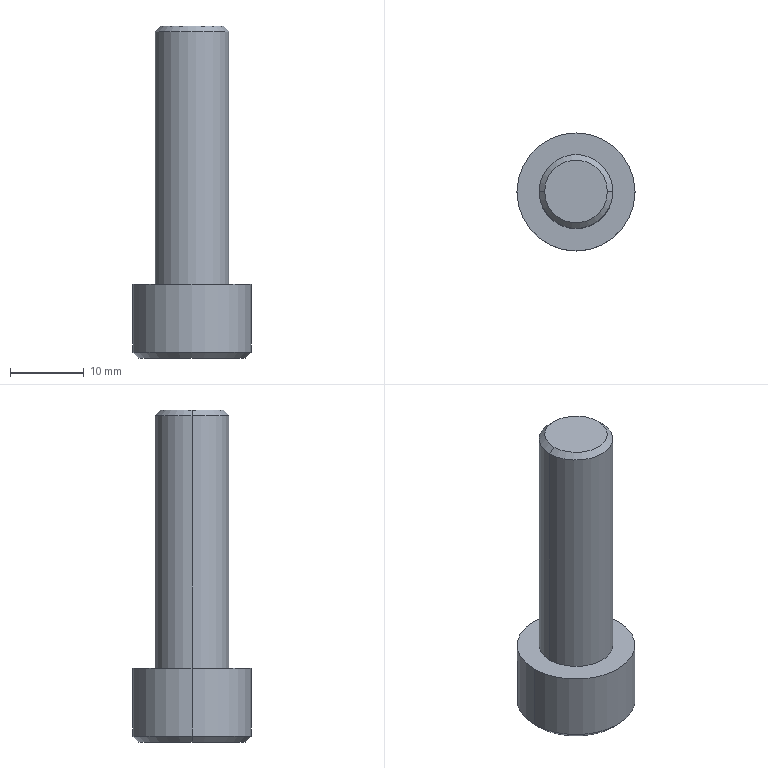Part | Creo | 1 solid | 18 faces | box 16 x 16 x 45 mm | volume 4403 mm3 | plane 10 | cylinder 4 | cone 4 | commonest cylinder face diameters 10 x2 16 x2
STEP:
#1=CARTESIAN_POINT('',(-123.202,226.324,-283.5));
#2=VERTEX_POINT('',#1);
#3=CARTESIAN_POINT('',(-107.202,226.324,-283.5));
#4=VERTEX_POINT('',#3);
#5=CARTESIAN_POINT('',(-115.202,226.324,-283.5));
#6=DIRECTION('',(0.,0.,1.));
#7=DIRECTION('',(-1.,0.,0.));
#8=AXIS2_PLACEMENT_3D('',#5,#6,#7);
#9=CIRCLE('',#8,8.);
#10=EDGE_CURVE('',#2,#4,#9,.T.);
#11=ORIENTED_EDGE('',*,*,#10,.F.);
#12=CARTESIAN_POINT('',(-115.202,226.324,-283.5));
#13=DIRECTION('',(0.,0.,1.));
#14=DIRECTION('',(1.,0.,0.));
#15=AXIS2_PLACEMENT_3D('',#12,#13,#14);
#16=CIRCLE('',#15,8.);
#17=EDGE_CURVE('',#4,#2,#16,.T.);
#18=ORIENTED_EDGE('',*,*,#17,.F.);
#19=EDGE_LOOP('',(#11,#18));
#20=FACE_OUTER_BOUND('',#19,.F.);
#21=CARTESIAN_POINT('',(-110.202,226.324,-283.5));
#22=VERTEX_POINT('',#21);
#23=CARTESIAN_POINT('',(-120.202,226.324,-283.5));
#24=VERTEX_POINT('',#23);
#25=CARTESIAN_POINT('',(-115.202,226.324,-283.5));
#26=DIRECTION('',(0.,0.,-1.));
#27=DIRECTION('',(1.,0.,0.));
#28=AXIS2_PLACEMENT_3D('',#25,#26,#27);
#29=CIRCLE('',#28,5.);
#30=EDGE_CURVE('',#22,#24,#29,.T.);
#31=ORIENTED_EDGE('',*,*,#30,.F.);
#32=CARTESIAN_POINT('',(-115.202,226.324,-283.5));
#33=DIRECTION('',(0.,0.,-1.));
#34=DIRECTION('',(-1.,0.,0.));
#35=AXIS2_PLACEMENT_3D('',#32,#33,#34);
#36=CIRCLE('',#35,5.);
#37=EDGE_CURVE('',#24,#22,#36,.T.);
#38=ORIENTED_EDGE('',*,*,#37,.F.);
#39=EDGE_LOOP('',(#31,#38));
#40=FACE_BOUND('',#39,.F.);
#41=CARTESIAN_POINT('',(-115.202,226.324,-283.5));
#42=DIRECTION('',(0.,0.,1.));
#43=DIRECTION('',(1.,0.,0.));
#44=AXIS2_PLACEMENT_3D('',#41,#42,#43);
#45=PLANE('',#44);
#46=ADVANCED_FACE('',(#20,#40),#45,.T.);
#47=CARTESIAN_POINT('',(-120.202,226.324,-249.25));
#48=VERTEX_POINT('',#47);
#49=CARTESIAN_POINT('',(-110.202,226.324,-249.25));
#50=VERTEX_POINT('',#49);
#51=CARTESIAN_POINT('',(-115.202,226.324,-249.25));
#52=DIRECTION('',(0.,0.,1.));
#53=DIRECTION('',(-1.,0.,0.));
#54=AXIS2_PLACEMENT_3D('',#51,#52,#53);
#55=CIRCLE('',#54,5.);
#56=EDGE_CURVE('',#48,#50,#55,.T.);
#57=ORIENTED_EDGE('',*,*,#56,.T.);
#58=CARTESIAN_POINT('',(-110.202,226.324,-283.5));
#59=DIRECTION('',(0.,0.,1.));
#60=VECTOR('',#59,34.25);
#61=LINE('',#58,#60);
#62=EDGE_CURVE('',#22,#50,#61,.T.);
#63=ORIENTED_EDGE('',*,*,#62,.F.);
#64=ORIENTED_EDGE('',*,*,#30,.T.);
#65=CARTESIAN_POINT('',(-120.202,226.324,-283.5));
#66=DIRECTION('',(0.,0.,1.));
#67=VECTOR('',#66,34.25);
#68=LINE('',#65,#67);
#69=EDGE_CURVE('',#24,#48,#68,.T.);
#70=ORIENTED_EDGE('',*,*,#69,.T.);
#71=EDGE_LOOP('',(#57,#63,#64,#70));
#72=FACE_OUTER_BOUND('',#71,.F.);
#73=CARTESIAN_POINT('',(-115.202,226.324,-295.5));
#74=DIRECTION('',(0.,0.,1.));
#75=DIRECTION('',(1.,0.,0.));
#76=AXIS2_PLACEMENT_3D('',#73,#74,#75);
#77=CYLINDRICAL_SURFACE('',#76,5.);
#78=ADVANCED_FACE('',(#72),#77,.T.);
#79=CARTESIAN_POINT('',(-119.452,226.324,-248.5));
#80=VERTEX_POINT('',#79);
#81=CARTESIAN_POINT('',(-110.952,226.324,-248.5));
#82=VERTEX_POINT('',#81);
#83=CARTESIAN_POINT('',(-115.202,226.324,-248.5));
#84=DIRECTION('',(0.,0.,1.));
#85=DIRECTION('',(-1.,0.,0.));
#86=AXIS2_PLACEMENT_3D('',#83,#84,#85);
#87=CIRCLE('',#86,4.25);
#88=EDGE_CURVE('',#80,#82,#87,.T.);
#89=ORIENTED_EDGE('',*,*,#88,.T.);
#90=CARTESIAN_POINT('',(-110.952,226.324,-248.5));
#91=DIRECTION('',(0.7071,0.,-0.7071));
#92=VECTOR('',#91,1.061);
#93=LINE('',#90,#92);
#94=EDGE_CURVE('',#82,#50,#93,.T.);
#95=ORIENTED_EDGE('',*,*,#94,.T.);
#96=ORIENTED_EDGE('',*,*,#56,.F.);
#97=CARTESIAN_POINT('',(-119.452,226.324,-248.5));
#98=DIRECTION('',(-0.7071,0.,-0.7071));
#99=VECTOR('',#98,1.061);
#100=LINE('',#97,#99);
#101=EDGE_CURVE('',#80,#48,#100,.T.);
#102=ORIENTED_EDGE('',*,*,#101,.F.);
#103=EDGE_LOOP('',(#89,#95,#96,#102));
#104=FACE_OUTER_BOUND('',#103,.F.);
#105=CARTESIAN_POINT('',(-115.202,226.324,-248.875));
#106=DIRECTION('',(0.,0.,-1.));
#107=DIRECTION('',(-1.,0.,0.));
#108=AXIS2_PLACEMENT_3D('',#105,#106,#107);
#109=CONICAL_SURFACE('',#108,4.625,45.);
#110=ADVANCED_FACE('',(#104),#109,.T.);
#111=CARTESIAN_POINT('',(-115.202,226.324,-248.5));
#112=DIRECTION('',(0.,0.,1.));
#113=DIRECTION('',(1.,0.,0.));
#114=AXIS2_PLACEMENT_3D('',#111,#112,#113);
#115=CIRCLE('',#114,4.25);
#116=EDGE_CURVE('',#82,#80,#115,.T.);
#117=ORIENTED_EDGE('',*,*,#116,.F.);
#118=ORIENTED_EDGE('',*,*,#88,.F.);
#119=EDGE_LOOP('',(#117,#118));
#120=FACE_OUTER_BOUND('',#119,.F.);
#121=CARTESIAN_POINT('',(-115.202,226.324,-248.5));
#122=DIRECTION('',(0.,0.,1.));
#123=DIRECTION('',(1.,0.,0.));
#124=AXIS2_PLACEMENT_3D('',#121,#122,#123);
#125=PLANE('',#124);
#126=ADVANCED_FACE('',(#120),#125,.T.);
#127=ORIENTED_EDGE('',*,*,#116,.T.);
#128=ORIENTED_EDGE('',*,*,#101,.T.);
#129=CARTESIAN_POINT('',(-115.202,226.324,-249.25));
#130=DIRECTION('',(0.,0.,1.));
#131=DIRECTION('',(1.,0.,0.));
#132=AXIS2_PLACEMENT_3D('',#129,#130,#131);
#133=CIRCLE('',#132,5.);
#134=EDGE_CURVE('',#50,#48,#133,.T.);
#135=ORIENTED_EDGE('',*,*,#134,.F.);
#136=ORIENTED_EDGE('',*,*,#94,.F.);
#137=EDGE_LOOP('',(#127,#128,#135,#136));
#138=FACE_OUTER_BOUND('',#137,.F.);
#139=CARTESIAN_POINT('',(-115.202,226.324,-248.875));
#140=DIRECTION('',(0.,0.,-1.));
#141=DIRECTION('',(-1.,0.,0.));
#142=AXIS2_PLACEMENT_3D('',#139,#140,#141);
#143=CONICAL_SURFACE('',#142,4.625,45.);
#144=ADVANCED_FACE('',(#138),#143,.T.);
#145=ORIENTED_EDGE('',*,*,#134,.T.);
#146=ORIENTED_EDGE('',*,*,#69,.F.);
#147=ORIENTED_EDGE('',*,*,#37,.T.);
#148=ORIENTED_EDGE('',*,*,#62,.T.);
#149=EDGE_LOOP('',(#145,#146,#147,#148));
#150=FACE_OUTER_BOUND('',#149,.F.);
#151=CARTESIAN_POINT('',(-115.202,226.324,-295.5));
#152=DIRECTION('',(0.,0.,1.));
#153=DIRECTION('',(1.,0.,0.));
#154=AXIS2_PLACEMENT_3D('',#151,#152,#153);
#155=CYLINDRICAL_SURFACE('',#154,5.);
#156=ADVANCED_FACE('',(#150),#155,.T.);
#157=CARTESIAN_POINT('',(-107.202,226.324,-292.7));
#158=VERTEX_POINT('',#157);
#159=CARTESIAN_POINT('',(-123.202,226.324,-292.7));
#160=VERTEX_POINT('',#159);
#161=CARTESIAN_POINT('',(-115.202,226.324,-292.7));
#162=DIRECTION('',(0.,0.,-1.));
#163=DIRECTION('',(1.,0.,0.));
#164=AXIS2_PLACEMENT_3D('',#161,#162,#163);
#165=CIRCLE('',#164,8.);
#166=EDGE_CURVE('',#158,#160,#165,.T.);
#167=ORIENTED_EDGE('',*,*,#166,.T.);
#168=CARTESIAN_POINT('',(-123.202,226.324,-292.7));
#169=DIRECTION('',(0.,0.,1.));
#170=VECTOR('',#169,9.2);
#171=LINE('',#168,#170);
#172=EDGE_CURVE('',#160,#2,#171,.T.);
#173=ORIENTED_EDGE('',*,*,#172,.T.);
#174=ORIENTED_EDGE('',*,*,#10,.T.);
#175=CARTESIAN_POINT('',(-107.202,226.324,-292.7));
#176=DIRECTION('',(0.,0.,1.));
#177=VECTOR('',#176,9.2);
#178=LINE('',#175,#177);
#179=EDGE_CURVE('',#158,#4,#178,.T.);
#180=ORIENTED_EDGE('',*,*,#179,.F.);
#181=EDGE_LOOP('',(#167,#173,#174,#180));
#182=FACE_OUTER_BOUND('',#181,.F.);
#183=CARTESIAN_POINT('',(-115.202,226.324,-295.5));
#184=DIRECTION('',(0.,0.,1.));
#185=DIRECTION('',(1.,0.,0.));
#186=AXIS2_PLACEMENT_3D('',#183,#184,#185);
#187=CYLINDRICAL_SURFACE('',#186,8.);
#188=ADVANCED_FACE('',(#182),#187,.T.);
#189=CARTESIAN_POINT('',(-108.002,226.324,-293.5));
#190=VERTEX_POINT('',#189);
#191=CARTESIAN_POINT('',(-122.402,226.324,-293.5));
#192=VERTEX_POINT('',#191);
#193=CARTESIAN_POINT('',(-115.202,226.324,-293.5));
#194=DIRECTION('',(0.,0.,-1.));
#195=DIRECTION('',(1.,0.,0.));
#196=AXIS2_PLACEMENT_3D('',#193,#194,#195);
#197=CIRCLE('',#196,7.2);
#198=EDGE_CURVE('',#190,#192,#197,.T.);
#199=ORIENTED_EDGE('',*,*,#198,.T.);
#200=CARTESIAN_POINT('',(-122.402,226.324,-293.5));
#201=DIRECTION('',(-0.7071,0.,0.7071));
#202=VECTOR('',#201,1.131);
#203=LINE('',#200,#202);
#204=EDGE_CURVE('',#192,#160,#203,.T.);
#205=ORIENTED_EDGE('',*,*,#204,.T.);
#206=ORIENTED_EDGE('',*,*,#166,.F.);
#207=CARTESIAN_POINT('',(-108.002,226.324,-293.5));
#208=DIRECTION('',(0.7071,0.,0.7071));
#209=VECTOR('',#208,1.131);
#210=LINE('',#207,#209);
#211=EDGE_CURVE('',#190,#158,#210,.T.);
#212=ORIENTED_EDGE('',*,*,#211,.F.);
#213=EDGE_LOOP('',(#199,#205,#206,#212));
#214=FACE_OUTER_BOUND('',#213,.F.);
#215=CARTESIAN_POINT('',(-115.202,226.324,-293.1));
#216=DIRECTION('',(0.,0.,1.));
#217=DIRECTION('',(1.,0.,0.));
#218=AXIS2_PLACEMENT_3D('',#215,#216,#217);
#219=CONICAL_SURFACE('',#218,7.6,45.);
#220=ADVANCED_FACE('',(#214),#219,.T.);
#221=ORIENTED_EDGE('',*,*,#198,.F.);
#222=CARTESIAN_POINT('',(-115.202,226.324,-293.5));
#223=DIRECTION('',(0.,0.,-1.));
#224=DIRECTION('',(-1.,0.,0.));
#225=AXIS2_PLACEMENT_3D('',#222,#223,#224);
#226=CIRCLE('',#225,7.2);
#227=EDGE_CURVE('',#192,#190,#226,.T.);
#228=ORIENTED_EDGE('',*,*,#227,.F.);
#229=EDGE_LOOP('',(#221,#228));
#230=FACE_OUTER_BOUND('',#229,.F.);
#231=CARTESIAN_POINT('',(-119.202,224.014,-293.5));
#232=VERTEX_POINT('',#231);
#233=CARTESIAN_POINT('',(-115.202,221.705,-293.5));
#234=VERTEX_POINT('',#233);
#235=CARTESIAN_POINT('',(-119.202,224.014,-293.5));
#236=DIRECTION('',(0.866,-0.5,0.));
#237=VECTOR('',#236,4.619);
#238=LINE('',#235,#237);
#239=EDGE_CURVE('',#232,#234,#238,.T.);
#240=ORIENTED_EDGE('',*,*,#239,.F.);
#241=CARTESIAN_POINT('',(-119.202,228.633,-293.5));
#242=VERTEX_POINT('',#241);
#243=CARTESIAN_POINT('',(-119.202,228.633,-293.5));
#244=DIRECTION('',(0.,-1.,0.));
#245=VECTOR('',#244,4.619);
#246=LINE('',#243,#245);
#247=EDGE_CURVE('',#242,#232,#246,.T.);
#248=ORIENTED_EDGE('',*,*,#247,.F.);
#249=CARTESIAN_POINT('',(-115.202,230.943,-293.5));
#250=VERTEX_POINT('',#249);
#251=CARTESIAN_POINT('',(-115.202,230.943,-293.5));
#252=DIRECTION('',(-0.866,-0.5,0.));
#253=VECTOR('',#252,4.619);
#254=LINE('',#251,#253);
#255=EDGE_CURVE('',#250,#242,#254,.T.);
#256=ORIENTED_EDGE('',*,*,#255,.F.);
#257=CARTESIAN_POINT('',(-111.202,228.633,-293.5));
#258=VERTEX_POINT('',#257);
#259=CARTESIAN_POINT('',(-111.202,228.633,-293.5));
#260=DIRECTION('',(-0.866,0.5,0.));
#261=VECTOR('',#260,4.619);
#262=LINE('',#259,#261);
#263=EDGE_CURVE('',#258,#250,#262,.T.);
#264=ORIENTED_EDGE('',*,*,#263,.F.);
#265=CARTESIAN_POINT('',(-111.202,224.014,-293.5));
#266=VERTEX_POINT('',#265);
#267=CARTESIAN_POINT('',(-111.202,224.014,-293.5));
#268=DIRECTION('',(0.,1.,0.));
#269=VECTOR('',#268,4.619);
#270=LINE('',#267,#269);
#271=EDGE_CURVE('',#266,#258,#270,.T.);
#272=ORIENTED_EDGE('',*,*,#271,.F.);
#273=CARTESIAN_POINT('',(-115.202,221.705,-293.5));
#274=DIRECTION('',(0.866,0.5,0.));
#275=VECTOR('',#274,4.619);
#276=LINE('',#273,#275);
#277=EDGE_CURVE('',#234,#266,#276,.T.);
#278=ORIENTED_EDGE('',*,*,#277,.F.);
#279=EDGE_LOOP('',(#240,#248,#256,#264,#272,#278));
#280=FACE_BOUND('',#279,.F.);
#281=CARTESIAN_POINT('',(-115.202,226.324,-293.5));
#282=DIRECTION('',(0.,0.,1.));
#283=DIRECTION('',(1.,0.,0.));
#284=AXIS2_PLACEMENT_3D('',#281,#282,#283);
#285=PLANE('',#284);
#286=ADVANCED_FACE('',(#230,#280),#285,.F.);
#287=ORIENTED_EDGE('',*,*,#227,.T.);
#288=ORIENTED_EDGE('',*,*,#211,.T.);
#289=CARTESIAN_POINT('',(-115.202,226.324,-292.7));
#290=DIRECTION('',(0.,0.,-1.));
#291=DIRECTION('',(-1.,0.,0.));
#292=AXIS2_PLACEMENT_3D('',#289,#290,#291);
#293=CIRCLE('',#292,8.);
#294=EDGE_CURVE('',#160,#158,#293,.T.);
#295=ORIENTED_EDGE('',*,*,#294,.F.);
#296=ORIENTED_EDGE('',*,*,#204,.F.);
#297=EDGE_LOOP('',(#287,#288,#295,#296));
#298=FACE_OUTER_BOUND('',#297,.F.);
#299=CARTESIAN_POINT('',(-115.202,226.324,-293.1));
#300=DIRECTION('',(0.,0.,1.));
#301=DIRECTION('',(1.,0.,0.));
#302=AXIS2_PLACEMENT_3D('',#299,#300,#301);
#303=CONICAL_SURFACE('',#302,7.6,45.);
#304=ADVANCED_FACE('',(#298),#303,.T.);
#305=ORIENTED_EDGE('',*,*,#294,.T.);
#306=ORIENTED_EDGE('',*,*,#179,.T.);
#307=ORIENTED_EDGE('',*,*,#17,.T.);
#308=ORIENTED_EDGE('',*,*,#172,.F.);
#309=EDGE_LOOP('',(#305,#306,#307,#308));
#310=FACE_OUTER_BOUND('',#309,.F.);
#311=CARTESIAN_POINT('',(-115.202,226.324,-295.5));
#312=DIRECTION('',(0.,0.,1.));
#313=DIRECTION('',(1.,0.,0.));
#314=AXIS2_PLACEMENT_3D('',#311,#312,#313);
#315=CYLINDRICAL_SURFACE('',#314,8.);
#316=ADVANCED_FACE('',(#310),#315,.T.);
#317=ORIENTED_EDGE('',*,*,#239,.T.);
#318=CARTESIAN_POINT('',(-115.202,221.705,-287.5));
#319=VERTEX_POINT('',#318);
#320=CARTESIAN_POINT('',(-115.202,221.705,-293.5));
#321=DIRECTION('',(0.,0.,1.));
#322=VECTOR('',#321,6.);
#323=LINE('',#320,#322);
#324=EDGE_CURVE('',#234,#319,#323,.T.);
#325=ORIENTED_EDGE('',*,*,#324,.T.);
#326=CARTESIAN_POINT('',(-119.202,224.014,-287.5));
#327=VERTEX_POINT('',#326);
#328=CARTESIAN_POINT('',(-115.202,221.705,-287.5));
#329=DIRECTION('',(-0.866,0.5,0.));
#330=VECTOR('',#329,4.619);
#331=LINE('',#328,#330);
#332=EDGE_CURVE('',#319,#327,#331,.T.);
#333=ORIENTED_EDGE('',*,*,#332,.T.);
#334=CARTESIAN_POINT('',(-119.202,224.014,-293.5));
#335=DIRECTION('',(0.,0.,1.));
#336=VECTOR('',#335,6.);
#337=LINE('',#334,#336);
#338=EDGE_CURVE('',#232,#327,#337,.T.);
#339=ORIENTED_EDGE('',*,*,#338,.F.);
#340=EDGE_LOOP('',(#317,#325,#333,#339));
#341=FACE_OUTER_BOUND('',#340,.F.);
#342=CARTESIAN_POINT('',(-115.202,221.705,-287.5));
#343=DIRECTION('',(-0.5,-0.866,0.));
#344=DIRECTION('',(0.866,-0.5,0.));
#345=AXIS2_PLACEMENT_3D('',#342,#343,#344);
#346=PLANE('',#345);
#347=ADVANCED_FACE('',(#341),#346,.F.);
#348=ORIENTED_EDGE('',*,*,#277,.T.);
#349=CARTESIAN_POINT('',(-111.202,224.014,-287.5));
#350=VERTEX_POINT('',#349);
#351=CARTESIAN_POINT('',(-111.202,224.014,-293.5));
#352=DIRECTION('',(0.,0.,1.));
#353=VECTOR('',#352,6.);
#354=LINE('',#351,#353);
#355=EDGE_CURVE('',#266,#350,#354,.T.);
#356=ORIENTED_EDGE('',*,*,#355,.T.);
#357=CARTESIAN_POINT('',(-111.202,224.014,-287.5));
#358=DIRECTION('',(-0.866,-0.5,0.));
#359=VECTOR('',#358,4.619);
#360=LINE('',#357,#359);
#361=EDGE_CURVE('',#350,#319,#360,.T.);
#362=ORIENTED_EDGE('',*,*,#361,.T.);
#363=ORIENTED_EDGE('',*,*,#324,.F.);
#364=EDGE_LOOP('',(#348,#356,#362,#363));
#365=FACE_OUTER_BOUND('',#364,.F.);
#366=CARTESIAN_POINT('',(-111.202,224.014,-287.5));
#367=DIRECTION('',(0.5,-0.866,0.));
#368=DIRECTION('',(0.866,0.5,0.));
#369=AXIS2_PLACEMENT_3D('',#366,#367,#368);
#370=PLANE('',#369);
#371=ADVANCED_FACE('',(#365),#370,.F.);
#372=ORIENTED_EDGE('',*,*,#271,.T.);
#373=CARTESIAN_POINT('',(-111.202,228.633,-287.5));
#374=VERTEX_POINT('',#373);
#375=CARTESIAN_POINT('',(-111.202,228.633,-293.5));
#376=DIRECTION('',(0.,0.,1.));
#377=VECTOR('',#376,6.);
#378=LINE('',#375,#377);
#379=EDGE_CURVE('',#258,#374,#378,.T.);
#380=ORIENTED_EDGE('',*,*,#379,.T.);
#381=CARTESIAN_POINT('',(-111.202,224.014,-287.5));
#382=DIRECTION('',(0.,1.,0.));
#383=VECTOR('',#382,4.619);
#384=LINE('',#381,#383);
#385=EDGE_CURVE('',#350,#374,#384,.T.);
#386=ORIENTED_EDGE('',*,*,#385,.F.);
#387=ORIENTED_EDGE('',*,*,#355,.F.);
#388=EDGE_LOOP('',(#372,#380,#386,#387));
#389=FACE_OUTER_BOUND('',#388,.F.);
#390=CARTESIAN_POINT('',(-111.202,228.633,-287.5));
#391=DIRECTION('',(1.,0.,0.));
#392=DIRECTION('',(0.,0.,-1.));
#393=AXIS2_PLACEMENT_3D('',#390,#391,#392);
#394=PLANE('',#393);
#395=ADVANCED_FACE('',(#389),#394,.F.);
#396=ORIENTED_EDGE('',*,*,#263,.T.);
#397=CARTESIAN_POINT('',(-115.202,230.943,-287.5));
#398=VERTEX_POINT('',#397);
#399=CARTESIAN_POINT('',(-115.202,230.943,-293.5));
#400=DIRECTION('',(0.,0.,1.));
#401=VECTOR('',#400,6.);
#402=LINE('',#399,#401);
#403=EDGE_CURVE('',#250,#398,#402,.T.);
#404=ORIENTED_EDGE('',*,*,#403,.T.);
#405=CARTESIAN_POINT('',(-115.202,230.943,-287.5));
#406=DIRECTION('',(0.866,-0.5,0.));
#407=VECTOR('',#406,4.619);
#408=LINE('',#405,#407);
#409=EDGE_CURVE('',#398,#374,#408,.T.);
#410=ORIENTED_EDGE('',*,*,#409,.T.);
#411=ORIENTED_EDGE('',*,*,#379,.F.);
#412=EDGE_LOOP('',(#396,#404,#410,#411));
#413=FACE_OUTER_BOUND('',#412,.F.);
#414=CARTESIAN_POINT('',(-115.202,230.943,-287.5));
#415=DIRECTION('',(0.5,0.866,0.));
#416=DIRECTION('',(-0.866,0.5,0.));
#417=AXIS2_PLACEMENT_3D('',#414,#415,#416);
#418=PLANE('',#417);
#419=ADVANCED_FACE('',(#413),#418,.F.);
#420=ORIENTED_EDGE('',*,*,#255,.T.);
#421=CARTESIAN_POINT('',(-119.202,228.633,-287.5));
#422=VERTEX_POINT('',#421);
#423=CARTESIAN_POINT('',(-119.202,228.633,-293.5));
#424=DIRECTION('',(0.,0.,1.));
#425=VECTOR('',#424,6.);
#426=LINE('',#423,#425);
#427=EDGE_CURVE('',#242,#422,#426,.T.);
#428=ORIENTED_EDGE('',*,*,#427,.T.);
#429=CARTESIAN_POINT('',(-119.202,228.633,-287.5));
#430=DIRECTION('',(0.866,0.5,0.));
#431=VECTOR('',#430,4.619);
#432=LINE('',#429,#431);
#433=EDGE_CURVE('',#422,#398,#432,.T.);
#434=ORIENTED_EDGE('',*,*,#433,.T.);
#435=ORIENTED_EDGE('',*,*,#403,.F.);
#436=EDGE_LOOP('',(#420,#428,#434,#435));
#437=FACE_OUTER_BOUND('',#436,.F.);
#438=CARTESIAN_POINT('',(-119.202,228.633,-287.5));
#439=DIRECTION('',(-0.5,0.866,0.));
#440=DIRECTION('',(-0.866,-0.5,0.));
#441=AXIS2_PLACEMENT_3D('',#438,#439,#440);
#442=PLANE('',#441);
#443=ADVANCED_FACE('',(#437),#442,.F.);
#444=ORIENTED_EDGE('',*,*,#247,.T.);
#445=ORIENTED_EDGE('',*,*,#338,.T.);
#446=CARTESIAN_POINT('',(-119.202,228.633,-287.5));
#447=DIRECTION('',(0.,-1.,0.));
#448=VECTOR('',#447,4.619);
#449=LINE('',#446,#448);
#450=EDGE_CURVE('',#422,#327,#449,.T.);
#451=ORIENTED_EDGE('',*,*,#450,.F.);
#452=ORIENTED_EDGE('',*,*,#427,.F.);
#453=EDGE_LOOP('',(#444,#445,#451,#452));
#454=FACE_OUTER_BOUND('',#453,.F.);
#455=CARTESIAN_POINT('',(-119.202,224.014,-287.5));
#456=DIRECTION('',(-1.,0.,0.));
#457=DIRECTION('',(0.,0.,1.));
#458=AXIS2_PLACEMENT_3D('',#455,#456,#457);
#459=PLANE('',#458);
#460=ADVANCED_FACE('',(#454),#459,.F.);
#461=ORIENTED_EDGE('',*,*,#361,.F.);
#462=ORIENTED_EDGE('',*,*,#385,.T.);
#463=ORIENTED_EDGE('',*,*,#409,.F.);
#464=ORIENTED_EDGE('',*,*,#433,.F.);
#465=ORIENTED_EDGE('',*,*,#450,.T.);
#466=ORIENTED_EDGE('',*,*,#332,.F.);
#467=EDGE_LOOP('',(#461,#462,#463,#464,#465,#466));
#468=FACE_OUTER_BOUND('',#467,.F.);
#469=CARTESIAN_POINT('',(-115.202,221.705,-287.5));
#470=DIRECTION('',(0.,0.,-1.));
#471=DIRECTION('',(-1.,0.,0.));
#472=AXIS2_PLACEMENT_3D('',#469,#470,#471);
#473=PLANE('',#472);
#474=ADVANCED_FACE('',(#468),#473,.T.);
#475=CLOSED_SHELL('',(#46,#78,#110,#126,#144,#156,#188,#220,#286,#304,#316,#347,#371,#395,#419,#443,#460,#474));
#476=MANIFOLD_SOLID_BREP('',#475);
#477=(LENGTH_UNIT()NAMED_UNIT(*)SI_UNIT(.MILLI.,.METRE.));
#478=UNCERTAINTY_MEASURE_WITH_UNIT(LENGTH_MEASURE(0.005037),#477,'','');
#479=(NAMED_UNIT(*)PLANE_ANGLE_UNIT()SI_UNIT($,.RADIAN.));
#480=PLANE_ANGLE_MEASURE_WITH_UNIT(PLANE_ANGLE_MEASURE(0.01745),#479);
#481=(CONVERSION_BASED_UNIT('DEGREE',#480)NAMED_UNIT(*)PLANE_ANGLE_UNIT());
#482=(NAMED_UNIT(*)SI_UNIT($,.STERADIAN.)SOLID_ANGLE_UNIT());
#483=(GEOMETRIC_REPRESENTATION_CONTEXT(3)GLOBAL_UNCERTAINTY_ASSIGNED_CONTEXT((#478))GLOBAL_UNIT_ASSIGNED_CONTEXT((#477,#481,#482))REPRESENTATION_CONTEXT('',''));
#484=ADVANCED_BREP_SHAPE_REPRESENTATION('',(#476),#483);